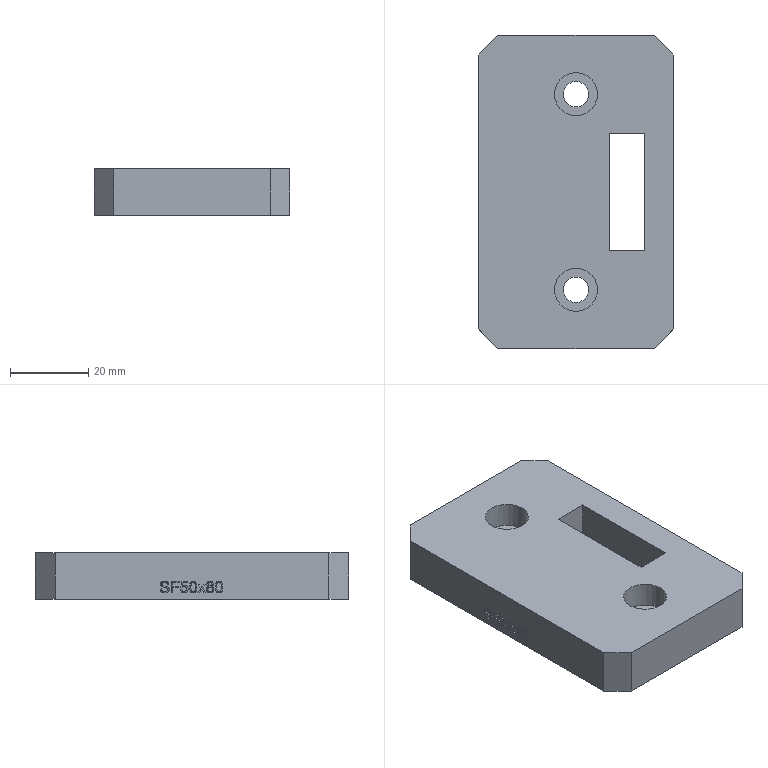Part | STEP file | lll_id390_x_t | 1 solid | 125 faces | box 50 x 80 x 12 mm | volume 42551 mm3 | other 62 | plane 59 | cylinder 4 | commonest cylinder face diameters 6.5 x2 11 x2